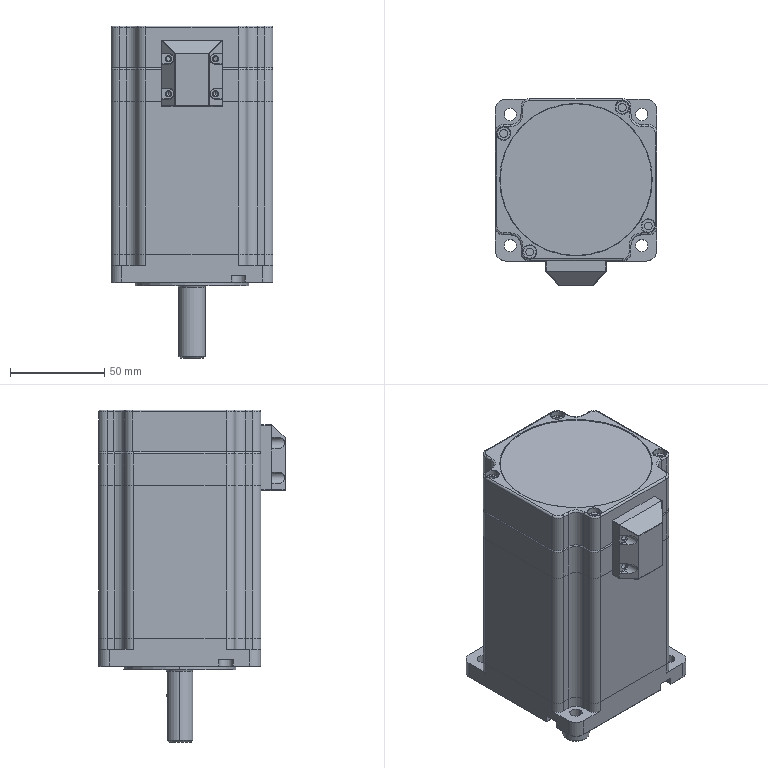Part | SolidWorks | features BaseBody 6 | 6 solids | 576 faces | box 85.85 x 99 x 176 mm | volume 601828 mm3 | cylinder 272 | plane 187 | torus 66 | cone 31 | spline 16 | sphere 4 | commonest cylinder face diameters 0.6 x58 8.9 x32 3.3 x24 11.4 x20 0.4 x16 6 x14